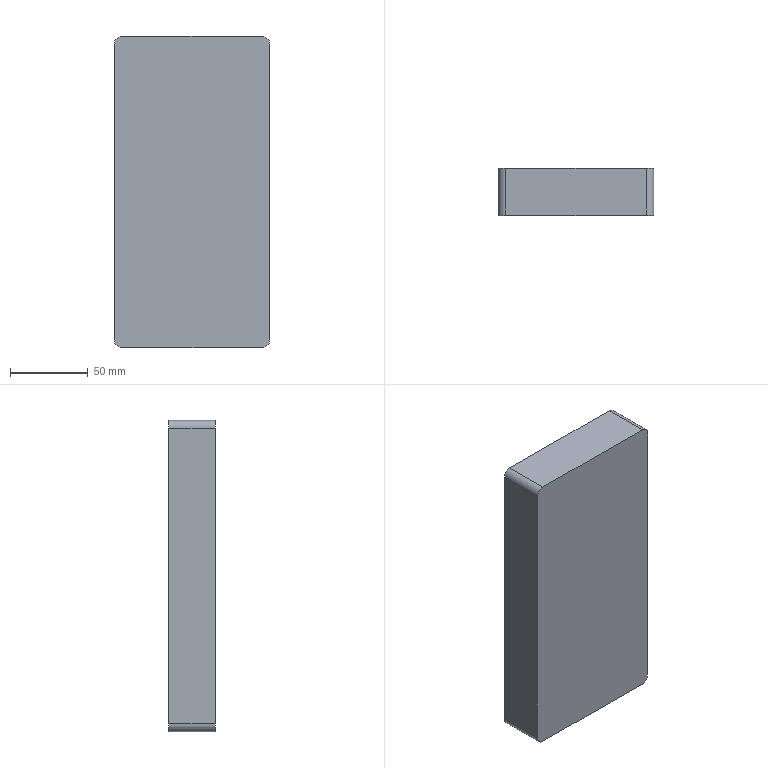Part | SolidWorks | features Extrusion 1, Fillet 1, ICE 1 | 1 solid | 247 faces | box 100 x 30 x 200 mm | volume 599338 mm3 | plane 186 | spline 57 | cylinder 4 | commonest cylinder face diameters 10 x4